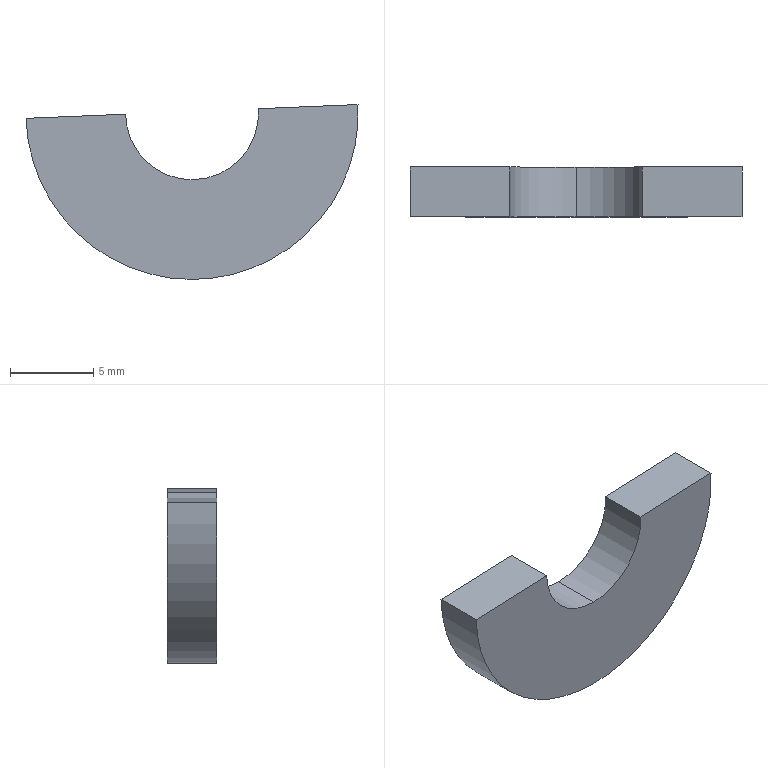Part | STEP file | Cuon T phu H01_8 | 1 solid | 8 faces | box 19.995 x 3 x 10.524 mm | volume 399.827 mm3 | cylinder 4 | plane 4 | commonest cylinder face diameters 8 x2 20 x2
STEP:
#1=CARTESIAN_POINT('',(0.,0.,0.));
#2=DIRECTION('',(0.,0.,1.));
#3=DIRECTION('',(1.,0.,0.));
#4=AXIS2_PLACEMENT_3D('',#1,#2,#3);
#5=CARTESIAN_POINT('',(3.99,3.,0.2758));
#6=VERTEX_POINT('',#5);
#7=CARTESIAN_POINT('',(3.99,0.,0.2758));
#8=VERTEX_POINT('',#7);
#9=CARTESIAN_POINT('',(3.99,3.,0.2758));
#10=DIRECTION('',(0.,-1.,0.));
#11=VECTOR('',#10,1.);
#12=LINE('',#9,#11);
#13=CARTESIAN_POINT('',(0.,3.,0.));
#14=DIRECTION('',(0.,-1.,0.));
#15=DIRECTION('',(0.,0.,-1.));
#16=AXIS2_PLACEMENT_3D('',#13,#14,#15);
#17=CYLINDRICAL_SURFACE('',#16,4.);
#18=CARTESIAN_POINT('',(1.64,0.));
#19=DIRECTION('',(0.,1.));
#20=VECTOR('',#19,1.);
#21=LINE('',#18,#20);
#22=(GEOMETRIC_REPRESENTATION_CONTEXT(2)PARAMETRIC_REPRESENTATION_CONTEXT()REPRESENTATION_CONTEXT('',''));
#23=DEFINITIONAL_REPRESENTATION('',(#21),#22);
#24=PCURVE('',#17,#23);
#25=CARTESIAN_POINT('',(-359.492,-20.57,-14.75));
#26=DIRECTION('',(0.0413,0.,-0.9991));
#27=DIRECTION('',(-0.9991,0.,-0.0413));
#28=AXIS2_PLACEMENT_3D('',#25,#26,#27);
#29=PLANE('',#28);
#30=CARTESIAN_POINT('',(-363.793,23.57));
#31=DIRECTION('',(0.,-1.));
#32=VECTOR('',#31,1.);
#33=LINE('',#30,#32);
#34=(GEOMETRIC_REPRESENTATION_CONTEXT(2)PARAMETRIC_REPRESENTATION_CONTEXT()REPRESENTATION_CONTEXT('',''));
#35=DEFINITIONAL_REPRESENTATION('',(#33),#34);
#36=PCURVE('',#29,#35);
#37=SURFACE_CURVE('',#12,(#24,#36),.PCURVE_S1.);
#38=EDGE_CURVE('',#6,#8,#37,.T.);
#39=ORIENTED_EDGE('',*,*,#38,.T.);
#40=CARTESIAN_POINT('',(0.,0.,-4.));
#41=VERTEX_POINT('',#40);
#42=CARTESIAN_POINT('',(0.,0.,0.));
#43=DIRECTION('',(0.,1.,0.));
#44=DIRECTION('',(0.,0.,1.));
#45=AXIS2_PLACEMENT_3D('',#42,#43,#44);
#46=CIRCLE('',#45,4.);
#47=CARTESIAN_POINT('',(3.142,3.));
#48=DIRECTION('',(-1.,0.));
#49=VECTOR('',#48,1.);
#50=LINE('',#47,#49);
#51=(GEOMETRIC_REPRESENTATION_CONTEXT(2)PARAMETRIC_REPRESENTATION_CONTEXT()REPRESENTATION_CONTEXT('',''));
#52=DEFINITIONAL_REPRESENTATION('',(#50),#51);
#53=PCURVE('',#17,#52);
#54=CARTESIAN_POINT('',(0.,0.,0.));
#55=DIRECTION('',(0.,1.,0.));
#56=DIRECTION('',(0.,0.,1.));
#57=AXIS2_PLACEMENT_3D('',#54,#55,#56);
#58=PLANE('',#57);
#59=CARTESIAN_POINT('',(0.,0.));
#60=DIRECTION('',(1.,0.));
#61=AXIS2_PLACEMENT_2D('',#59,#60);
#62=CIRCLE('',#61,4.);
#63=(GEOMETRIC_REPRESENTATION_CONTEXT(2)PARAMETRIC_REPRESENTATION_CONTEXT()REPRESENTATION_CONTEXT('',''));
#64=DEFINITIONAL_REPRESENTATION('',(#62),#63);
#65=PCURVE('',#58,#64);
#66=SURFACE_CURVE('',#46,(#53,#65),.PCURVE_S1.);
#67=EDGE_CURVE('',#8,#41,#66,.T.);
#68=ORIENTED_EDGE('',*,*,#67,.T.);
#69=CARTESIAN_POINT('',(0.,3.,-4.));
#70=VERTEX_POINT('',#69);
#71=CARTESIAN_POINT('',(0.,3.,-4.));
#72=DIRECTION('',(0.,-1.,0.));
#73=VECTOR('',#72,1.);
#74=LINE('',#71,#73);
#75=CARTESIAN_POINT('',(0.,0.));
#76=DIRECTION('',(0.,1.));
#77=VECTOR('',#76,1.);
#78=LINE('',#75,#77);
#79=(GEOMETRIC_REPRESENTATION_CONTEXT(2)PARAMETRIC_REPRESENTATION_CONTEXT()REPRESENTATION_CONTEXT('',''));
#80=DEFINITIONAL_REPRESENTATION('',(#78),#79);
#81=PCURVE('',#17,#80);
#82=CARTESIAN_POINT('',(0.,3.,0.));
#83=DIRECTION('',(0.,-1.,0.));
#84=DIRECTION('',(0.,0.,-1.));
#85=AXIS2_PLACEMENT_3D('',#82,#83,#84);
#86=CYLINDRICAL_SURFACE('',#85,4.);
#87=CARTESIAN_POINT('',(6.283,0.));
#88=DIRECTION('',(0.,1.));
#89=VECTOR('',#88,1.);
#90=LINE('',#87,#89);
#91=(GEOMETRIC_REPRESENTATION_CONTEXT(2)PARAMETRIC_REPRESENTATION_CONTEXT()REPRESENTATION_CONTEXT('',''));
#92=DEFINITIONAL_REPRESENTATION('',(#90),#91);
#93=PCURVE('',#86,#92);
#94=SURFACE_CURVE('',#74,(#81,#93),.PCURVE_S1.);
#95=EDGE_CURVE('',#70,#41,#94,.T.);
#96=ORIENTED_EDGE('',*,*,#95,.F.);
#97=CARTESIAN_POINT('',(0.,3.,0.));
#98=DIRECTION('',(0.,1.,0.));
#99=DIRECTION('',(0.,0.,1.));
#100=AXIS2_PLACEMENT_3D('',#97,#98,#99);
#101=CIRCLE('',#100,4.);
#102=CARTESIAN_POINT('',(3.142,0.));
#103=DIRECTION('',(-1.,0.));
#104=VECTOR('',#103,1.);
#105=LINE('',#102,#104);
#106=(GEOMETRIC_REPRESENTATION_CONTEXT(2)PARAMETRIC_REPRESENTATION_CONTEXT()REPRESENTATION_CONTEXT('',''));
#107=DEFINITIONAL_REPRESENTATION('',(#105),#106);
#108=PCURVE('',#17,#107);
#109=CARTESIAN_POINT('',(0.,3.,0.));
#110=DIRECTION('',(0.,1.,0.));
#111=DIRECTION('',(0.,0.,1.));
#112=AXIS2_PLACEMENT_3D('',#109,#110,#111);
#113=PLANE('',#112);
#114=CARTESIAN_POINT('',(0.,0.));
#115=DIRECTION('',(1.,0.));
#116=AXIS2_PLACEMENT_2D('',#114,#115);
#117=CIRCLE('',#116,4.);
#118=(GEOMETRIC_REPRESENTATION_CONTEXT(2)PARAMETRIC_REPRESENTATION_CONTEXT()REPRESENTATION_CONTEXT('',''));
#119=DEFINITIONAL_REPRESENTATION('',(#117),#118);
#120=PCURVE('',#113,#119);
#121=SURFACE_CURVE('',#101,(#108,#120),.PCURVE_S1.);
#122=EDGE_CURVE('',#6,#70,#121,.T.);
#123=ORIENTED_EDGE('',*,*,#122,.F.);
#124=EDGE_LOOP('',(#39,#68,#96,#123));
#125=FACE_BOUND('',#124,.F.);
#126=ADVANCED_FACE('',(#125),#17,.F.);
#127=CARTESIAN_POINT('',(0.,3.,-10.));
#128=VERTEX_POINT('',#127);
#129=CARTESIAN_POINT('',(-9.995,3.,-0.3024));
#130=VERTEX_POINT('',#129);
#131=CARTESIAN_POINT('',(0.,3.,0.));
#132=DIRECTION('',(0.,1.,0.));
#133=DIRECTION('',(0.,0.,1.));
#134=AXIS2_PLACEMENT_3D('',#131,#132,#133);
#135=CIRCLE('',#134,10.);
#136=CARTESIAN_POINT('',(0.,3.,0.));
#137=DIRECTION('',(0.,-1.,0.));
#138=DIRECTION('',(0.,0.,-1.));
#139=AXIS2_PLACEMENT_3D('',#136,#137,#138);
#140=CYLINDRICAL_SURFACE('',#139,10.);
#141=CARTESIAN_POINT('',(9.425,0.));
#142=DIRECTION('',(-1.,0.));
#143=VECTOR('',#142,1.);
#144=LINE('',#141,#143);
#145=(GEOMETRIC_REPRESENTATION_CONTEXT(2)PARAMETRIC_REPRESENTATION_CONTEXT()REPRESENTATION_CONTEXT('',''));
#146=DEFINITIONAL_REPRESENTATION('',(#144),#145);
#147=PCURVE('',#140,#146);
#148=CARTESIAN_POINT('',(0.,0.));
#149=DIRECTION('',(1.,0.));
#150=AXIS2_PLACEMENT_2D('',#148,#149);
#151=CIRCLE('',#150,10.);
#152=(GEOMETRIC_REPRESENTATION_CONTEXT(2)PARAMETRIC_REPRESENTATION_CONTEXT()REPRESENTATION_CONTEXT('',''));
#153=DEFINITIONAL_REPRESENTATION('',(#151),#152);
#154=PCURVE('',#113,#153);
#155=SURFACE_CURVE('',#135,(#147,#154),.PCURVE_S1.);
#156=EDGE_CURVE('',#128,#130,#155,.T.);
#157=ORIENTED_EDGE('',*,*,#156,.F.);
#158=CARTESIAN_POINT('',(0.,0.,-10.));
#159=VERTEX_POINT('',#158);
#160=CARTESIAN_POINT('',(0.,3.,-10.));
#161=DIRECTION('',(0.,-1.,0.));
#162=VECTOR('',#161,1.);
#163=LINE('',#160,#162);
#164=CARTESIAN_POINT('',(6.283,0.));
#165=DIRECTION('',(0.,1.));
#166=VECTOR('',#165,1.);
#167=LINE('',#164,#166);
#168=(GEOMETRIC_REPRESENTATION_CONTEXT(2)PARAMETRIC_REPRESENTATION_CONTEXT()REPRESENTATION_CONTEXT('',''));
#169=DEFINITIONAL_REPRESENTATION('',(#167),#168);
#170=PCURVE('',#140,#169);
#171=CARTESIAN_POINT('',(0.,3.,0.));
#172=DIRECTION('',(0.,-1.,0.));
#173=DIRECTION('',(0.,0.,-1.));
#174=AXIS2_PLACEMENT_3D('',#171,#172,#173);
#175=CYLINDRICAL_SURFACE('',#174,10.);
#176=CARTESIAN_POINT('',(0.,0.));
#177=DIRECTION('',(0.,1.));
#178=VECTOR('',#177,1.);
#179=LINE('',#176,#178);
#180=(GEOMETRIC_REPRESENTATION_CONTEXT(2)PARAMETRIC_REPRESENTATION_CONTEXT()REPRESENTATION_CONTEXT('',''));
#181=DEFINITIONAL_REPRESENTATION('',(#179),#180);
#182=PCURVE('',#175,#181);
#183=SURFACE_CURVE('',#163,(#170,#182),.PCURVE_S1.);
#184=EDGE_CURVE('',#128,#159,#183,.T.);
#185=ORIENTED_EDGE('',*,*,#184,.T.);
#186=CARTESIAN_POINT('',(-9.995,0.,-0.3024));
#187=VERTEX_POINT('',#186);
#188=CARTESIAN_POINT('',(0.,0.,0.));
#189=DIRECTION('',(0.,1.,0.));
#190=DIRECTION('',(0.,0.,1.));
#191=AXIS2_PLACEMENT_3D('',#188,#189,#190);
#192=CIRCLE('',#191,10.);
#193=CARTESIAN_POINT('',(9.425,3.));
#194=DIRECTION('',(-1.,0.));
#195=VECTOR('',#194,1.);
#196=LINE('',#193,#195);
#197=(GEOMETRIC_REPRESENTATION_CONTEXT(2)PARAMETRIC_REPRESENTATION_CONTEXT()REPRESENTATION_CONTEXT('',''));
#198=DEFINITIONAL_REPRESENTATION('',(#196),#197);
#199=PCURVE('',#140,#198);
#200=CARTESIAN_POINT('',(0.,0.));
#201=DIRECTION('',(1.,0.));
#202=AXIS2_PLACEMENT_2D('',#200,#201);
#203=CIRCLE('',#202,10.);
#204=(GEOMETRIC_REPRESENTATION_CONTEXT(2)PARAMETRIC_REPRESENTATION_CONTEXT()REPRESENTATION_CONTEXT('',''));
#205=DEFINITIONAL_REPRESENTATION('',(#203),#204);
#206=PCURVE('',#58,#205);
#207=SURFACE_CURVE('',#192,(#199,#206),.PCURVE_S1.);
#208=EDGE_CURVE('',#159,#187,#207,.T.);
#209=ORIENTED_EDGE('',*,*,#208,.T.);
#210=CARTESIAN_POINT('',(-9.995,3.,-0.3024));
#211=DIRECTION('',(0.,1.,0.));
#212=VECTOR('',#211,1.);
#213=LINE('',#210,#212);
#214=CARTESIAN_POINT('',(4.743,0.));
#215=DIRECTION('',(0.,-1.));
#216=VECTOR('',#215,1.);
#217=LINE('',#214,#216);
#218=(GEOMETRIC_REPRESENTATION_CONTEXT(2)PARAMETRIC_REPRESENTATION_CONTEXT()REPRESENTATION_CONTEXT('',''));
#219=DEFINITIONAL_REPRESENTATION('',(#217),#218);
#220=PCURVE('',#140,#219);
#221=CARTESIAN_POINT('',(-359.492,-20.57,-14.75));
#222=DIRECTION('',(0.0413,0.,-0.9991));
#223=DIRECTION('',(-0.9991,0.,-0.0413));
#224=AXIS2_PLACEMENT_3D('',#221,#222,#223);
#225=PLANE('',#224);
#226=CARTESIAN_POINT('',(-349.795,23.57));
#227=DIRECTION('',(0.,1.));
#228=VECTOR('',#227,1.);
#229=LINE('',#226,#228);
#230=(GEOMETRIC_REPRESENTATION_CONTEXT(2)PARAMETRIC_REPRESENTATION_CONTEXT()REPRESENTATION_CONTEXT('',''));
#231=DEFINITIONAL_REPRESENTATION('',(#229),#230);
#232=PCURVE('',#225,#231);
#233=SURFACE_CURVE('',#213,(#220,#232),.PCURVE_S1.);
#234=EDGE_CURVE('',#187,#130,#233,.T.);
#235=ORIENTED_EDGE('',*,*,#234,.T.);
#236=EDGE_LOOP('',(#157,#185,#209,#235));
#237=FACE_BOUND('',#236,.T.);
#238=ADVANCED_FACE('',(#237),#140,.T.);
#239=CARTESIAN_POINT('',(9.986,3.,0.5237));
#240=VERTEX_POINT('',#239);
#241=CARTESIAN_POINT('',(-0.004574,3.,0.1106));
#242=DIRECTION('',(-0.9991,0.,-0.0413));
#243=VECTOR('',#242,1.);
#244=LINE('',#241,#243);
#245=CARTESIAN_POINT('',(0.1106,-0.004574));
#246=DIRECTION('',(-0.0413,-0.9991));
#247=VECTOR('',#246,1.);
#248=LINE('',#245,#247);
#249=(GEOMETRIC_REPRESENTATION_CONTEXT(2)PARAMETRIC_REPRESENTATION_CONTEXT()REPRESENTATION_CONTEXT('',''));
#250=DEFINITIONAL_REPRESENTATION('',(#248),#249);
#251=PCURVE('',#113,#250);
#252=CARTESIAN_POINT('',(-359.795,23.57));
#253=DIRECTION('',(1.,0.));
#254=VECTOR('',#253,1.);
#255=LINE('',#252,#254);
#256=(GEOMETRIC_REPRESENTATION_CONTEXT(2)PARAMETRIC_REPRESENTATION_CONTEXT()REPRESENTATION_CONTEXT('',''));
#257=DEFINITIONAL_REPRESENTATION('',(#255),#256);
#258=PCURVE('',#29,#257);
#259=SURFACE_CURVE('',#244,(#251,#258),.PCURVE_S1.);
#260=EDGE_CURVE('',#240,#6,#259,.T.);
#261=ORIENTED_EDGE('',*,*,#260,.F.);
#262=CARTESIAN_POINT('',(0.,3.,0.));
#263=DIRECTION('',(0.,1.,0.));
#264=DIRECTION('',(0.,0.,1.));
#265=AXIS2_PLACEMENT_3D('',#262,#263,#264);
#266=CIRCLE('',#265,10.);
#267=CARTESIAN_POINT('',(0.,0.));
#268=DIRECTION('',(1.,0.));
#269=AXIS2_PLACEMENT_2D('',#267,#268);
#270=CIRCLE('',#269,10.);
#271=(GEOMETRIC_REPRESENTATION_CONTEXT(2)PARAMETRIC_REPRESENTATION_CONTEXT()REPRESENTATION_CONTEXT('',''));
#272=DEFINITIONAL_REPRESENTATION('',(#270),#271);
#273=PCURVE('',#113,#272);
#274=CARTESIAN_POINT('',(3.142,0.));
#275=DIRECTION('',(-1.,0.));
#276=VECTOR('',#275,1.);
#277=LINE('',#274,#276);
#278=(GEOMETRIC_REPRESENTATION_CONTEXT(2)PARAMETRIC_REPRESENTATION_CONTEXT()REPRESENTATION_CONTEXT('',''));
#279=DEFINITIONAL_REPRESENTATION('',(#277),#278);
#280=PCURVE('',#175,#279);
#281=SURFACE_CURVE('',#266,(#273,#280),.PCURVE_S1.);
#282=EDGE_CURVE('',#240,#128,#281,.T.);
#283=ORIENTED_EDGE('',*,*,#282,.T.);
#284=ORIENTED_EDGE('',*,*,#156,.T.);
#285=CARTESIAN_POINT('',(-4.,3.,-0.05451));
#286=VERTEX_POINT('',#285);
#287=CARTESIAN_POINT('',(-0.004574,3.,0.1106));
#288=DIRECTION('',(-0.9991,0.,-0.0413));
#289=VECTOR('',#288,1.);
#290=LINE('',#287,#289);
#291=CARTESIAN_POINT('',(0.1106,-0.004574));
#292=DIRECTION('',(-0.0413,-0.9991));
#293=VECTOR('',#292,1.);
#294=LINE('',#291,#293);
#295=(GEOMETRIC_REPRESENTATION_CONTEXT(2)PARAMETRIC_REPRESENTATION_CONTEXT()REPRESENTATION_CONTEXT('',''));
#296=DEFINITIONAL_REPRESENTATION('',(#294),#295);
#297=PCURVE('',#113,#296);
#298=CARTESIAN_POINT('',(-359.795,23.57));
#299=DIRECTION('',(1.,0.));
#300=VECTOR('',#299,1.);
#301=LINE('',#298,#300);
#302=(GEOMETRIC_REPRESENTATION_CONTEXT(2)PARAMETRIC_REPRESENTATION_CONTEXT()REPRESENTATION_CONTEXT('',''));
#303=DEFINITIONAL_REPRESENTATION('',(#301),#302);
#304=PCURVE('',#225,#303);
#305=SURFACE_CURVE('',#290,(#297,#304),.PCURVE_S1.);
#306=EDGE_CURVE('',#286,#130,#305,.T.);
#307=ORIENTED_EDGE('',*,*,#306,.F.);
#308=CARTESIAN_POINT('',(0.,3.,0.));
#309=DIRECTION('',(0.,1.,0.));
#310=DIRECTION('',(0.,0.,1.));
#311=AXIS2_PLACEMENT_3D('',#308,#309,#310);
#312=CIRCLE('',#311,4.);
#313=CARTESIAN_POINT('',(0.,0.));
#314=DIRECTION('',(1.,0.));
#315=AXIS2_PLACEMENT_2D('',#313,#314);
#316=CIRCLE('',#315,4.);
#317=(GEOMETRIC_REPRESENTATION_CONTEXT(2)PARAMETRIC_REPRESENTATION_CONTEXT()REPRESENTATION_CONTEXT('',''));
#318=DEFINITIONAL_REPRESENTATION('',(#316),#317);
#319=PCURVE('',#113,#318);
#320=CARTESIAN_POINT('',(9.425,0.));
#321=DIRECTION('',(-1.,0.));
#322=VECTOR('',#321,1.);
#323=LINE('',#320,#322);
#324=(GEOMETRIC_REPRESENTATION_CONTEXT(2)PARAMETRIC_REPRESENTATION_CONTEXT()REPRESENTATION_CONTEXT('',''));
#325=DEFINITIONAL_REPRESENTATION('',(#323),#324);
#326=PCURVE('',#86,#325);
#327=SURFACE_CURVE('',#312,(#319,#326),.PCURVE_S1.);
#328=EDGE_CURVE('',#70,#286,#327,.T.);
#329=ORIENTED_EDGE('',*,*,#328,.F.);
#330=ORIENTED_EDGE('',*,*,#122,.F.);
#331=EDGE_LOOP('',(#261,#283,#284,#307,#329,#330));
#332=FACE_BOUND('',#331,.T.);
#333=ADVANCED_FACE('',(#332),#113,.T.);
#334=CARTESIAN_POINT('',(9.986,0.,0.5237));
#335=VERTEX_POINT('',#334);
#336=CARTESIAN_POINT('',(0.,0.,0.));
#337=DIRECTION('',(0.,1.,0.));
#338=DIRECTION('',(0.,0.,1.));
#339=AXIS2_PLACEMENT_3D('',#336,#337,#338);
#340=CIRCLE('',#339,10.);
#341=CARTESIAN_POINT('',(0.,0.));
#342=DIRECTION('',(1.,0.));
#343=AXIS2_PLACEMENT_2D('',#341,#342);
#344=CIRCLE('',#343,10.);
#345=(GEOMETRIC_REPRESENTATION_CONTEXT(2)PARAMETRIC_REPRESENTATION_CONTEXT()REPRESENTATION_CONTEXT('',''));
#346=DEFINITIONAL_REPRESENTATION('',(#344),#345);
#347=PCURVE('',#58,#346);
#348=CARTESIAN_POINT('',(3.142,3.));
#349=DIRECTION('',(-1.,0.));
#350=VECTOR('',#349,1.);
#351=LINE('',#348,#350);
#352=(GEOMETRIC_REPRESENTATION_CONTEXT(2)PARAMETRIC_REPRESENTATION_CONTEXT()REPRESENTATION_CONTEXT('',''));
#353=DEFINITIONAL_REPRESENTATION('',(#351),#352);
#354=PCURVE('',#175,#353);
#355=SURFACE_CURVE('',#340,(#347,#354),.PCURVE_S1.);
#356=EDGE_CURVE('',#335,#159,#355,.T.);
#357=ORIENTED_EDGE('',*,*,#356,.F.);
#358=CARTESIAN_POINT('',(-0.004574,0.,0.1106));
#359=DIRECTION('',(-0.9991,0.,-0.0413));
#360=VECTOR('',#359,1.);
#361=LINE('',#358,#360);
#362=CARTESIAN_POINT('',(0.1106,-0.004574));
#363=DIRECTION('',(-0.0413,-0.9991));
#364=VECTOR('',#363,1.);
#365=LINE('',#362,#364);
#366=(GEOMETRIC_REPRESENTATION_CONTEXT(2)PARAMETRIC_REPRESENTATION_CONTEXT()REPRESENTATION_CONTEXT('',''));
#367=DEFINITIONAL_REPRESENTATION('',(#365),#366);
#368=PCURVE('',#58,#367);
#369=CARTESIAN_POINT('',(-359.795,20.57));
#370=DIRECTION('',(1.,0.));
#371=VECTOR('',#370,1.);
#372=LINE('',#369,#371);
#373=(GEOMETRIC_REPRESENTATION_CONTEXT(2)PARAMETRIC_REPRESENTATION_CONTEXT()REPRESENTATION_CONTEXT('',''));
#374=DEFINITIONAL_REPRESENTATION('',(#372),#373);
#375=PCURVE('',#29,#374);
#376=SURFACE_CURVE('',#361,(#368,#375),.PCURVE_S1.);
#377=EDGE_CURVE('',#335,#8,#376,.T.);
#378=ORIENTED_EDGE('',*,*,#377,.T.);
#379=ORIENTED_EDGE('',*,*,#67,.T.);
#380=CARTESIAN_POINT('',(-4.,0.,-0.05451));
#381=VERTEX_POINT('',#380);
#382=CARTESIAN_POINT('',(0.,0.,0.));
#383=DIRECTION('',(0.,1.,0.));
#384=DIRECTION('',(0.,0.,1.));
#385=AXIS2_PLACEMENT_3D('',#382,#383,#384);
#386=CIRCLE('',#385,4.);
#387=CARTESIAN_POINT('',(0.,0.));
#388=DIRECTION('',(1.,0.));
#389=AXIS2_PLACEMENT_2D('',#387,#388);
#390=CIRCLE('',#389,4.);
#391=(GEOMETRIC_REPRESENTATION_CONTEXT(2)PARAMETRIC_REPRESENTATION_CONTEXT()REPRESENTATION_CONTEXT('',''));
#392=DEFINITIONAL_REPRESENTATION('',(#390),#391);
#393=PCURVE('',#58,#392);
#394=CARTESIAN_POINT('',(9.425,3.));
#395=DIRECTION('',(-1.,0.));
#396=VECTOR('',#395,1.);
#397=LINE('',#394,#396);
#398=(GEOMETRIC_REPRESENTATION_CONTEXT(2)PARAMETRIC_REPRESENTATION_CONTEXT()REPRESENTATION_CONTEXT('',''));
#399=DEFINITIONAL_REPRESENTATION('',(#397),#398);
#400=PCURVE('',#86,#399);
#401=SURFACE_CURVE('',#386,(#393,#400),.PCURVE_S1.);
#402=EDGE_CURVE('',#41,#381,#401,.T.);
#403=ORIENTED_EDGE('',*,*,#402,.T.);
#404=CARTESIAN_POINT('',(-0.004574,0.,0.1106));
#405=DIRECTION('',(-0.9991,0.,-0.0413));
#406=VECTOR('',#405,1.);
#407=LINE('',#404,#406);
#408=CARTESIAN_POINT('',(0.1106,-0.004574));
#409=DIRECTION('',(-0.0413,-0.9991));
#410=VECTOR('',#409,1.);
#411=LINE('',#408,#410);
#412=(GEOMETRIC_REPRESENTATION_CONTEXT(2)PARAMETRIC_REPRESENTATION_CONTEXT()REPRESENTATION_CONTEXT('',''));
#413=DEFINITIONAL_REPRESENTATION('',(#411),#412);
#414=PCURVE('',#58,#413);
#415=CARTESIAN_POINT('',(-359.795,20.57));
#416=DIRECTION('',(1.,0.));
#417=VECTOR('',#416,1.);
#418=LINE('',#415,#417);
#419=(GEOMETRIC_REPRESENTATION_CONTEXT(2)PARAMETRIC_REPRESENTATION_CONTEXT()REPRESENTATION_CONTEXT('',''));
#420=DEFINITIONAL_REPRESENTATION('',(#418),#419);
#421=PCURVE('',#225,#420);
#422=SURFACE_CURVE('',#407,(#414,#421),.PCURVE_S1.);
#423=EDGE_CURVE('',#381,#187,#422,.T.);
#424=ORIENTED_EDGE('',*,*,#423,.T.);
#425=ORIENTED_EDGE('',*,*,#208,.F.);
#426=EDGE_LOOP('',(#357,#378,#379,#403,#424,#425));
#427=FACE_BOUND('',#426,.T.);
#428=ADVANCED_FACE('',(#427),#58,.F.);
#429=ORIENTED_EDGE('',*,*,#184,.F.);
#430=ORIENTED_EDGE('',*,*,#282,.F.);
#431=CARTESIAN_POINT('',(9.986,3.,0.5237));
#432=DIRECTION('',(0.,-1.,0.));
#433=VECTOR('',#432,1.);
#434=LINE('',#431,#433);
#435=CARTESIAN_POINT('',(1.623,0.));
#436=DIRECTION('',(0.,1.));
#437=VECTOR('',#436,1.);
#438=LINE('',#435,#437);
#439=(GEOMETRIC_REPRESENTATION_CONTEXT(2)PARAMETRIC_REPRESENTATION_CONTEXT()REPRESENTATION_CONTEXT('',''));
#440=DEFINITIONAL_REPRESENTATION('',(#438),#439);
#441=PCURVE('',#175,#440);
#442=CARTESIAN_POINT('',(-369.794,23.57));
#443=DIRECTION('',(0.,-1.));
#444=VECTOR('',#443,1.);
#445=LINE('',#442,#444);
#446=(GEOMETRIC_REPRESENTATION_CONTEXT(2)PARAMETRIC_REPRESENTATION_CONTEXT()REPRESENTATION_CONTEXT('',''));
#447=DEFINITIONAL_REPRESENTATION('',(#445),#446);
#448=PCURVE('',#29,#447);
#449=SURFACE_CURVE('',#434,(#441,#448),.PCURVE_S1.);
#450=EDGE_CURVE('',#240,#335,#449,.T.);
#451=ORIENTED_EDGE('',*,*,#450,.T.);
#452=ORIENTED_EDGE('',*,*,#356,.T.);
#453=EDGE_LOOP('',(#429,#430,#451,#452));
#454=FACE_BOUND('',#453,.T.);
#455=ADVANCED_FACE('',(#454),#175,.T.);
#456=ORIENTED_EDGE('',*,*,#402,.T.);
#457=CARTESIAN_POINT('',(-4.,3.,-0.05451));
#458=DIRECTION('',(0.,1.,0.));
#459=VECTOR('',#458,1.);
#460=LINE('',#457,#459);
#461=CARTESIAN_POINT('',(4.726,0.));
#462=DIRECTION('',(0.,-1.));
#463=VECTOR('',#462,1.);
#464=LINE('',#461,#463);
#465=(GEOMETRIC_REPRESENTATION_CONTEXT(2)PARAMETRIC_REPRESENTATION_CONTEXT()REPRESENTATION_CONTEXT('',''));
#466=DEFINITIONAL_REPRESENTATION('',(#464),#465);
#467=PCURVE('',#86,#466);
#468=CARTESIAN_POINT('',(-355.796,23.57));
#469=DIRECTION('',(0.,1.));
#470=VECTOR('',#469,1.);
#471=LINE('',#468,#470);
#472=(GEOMETRIC_REPRESENTATION_CONTEXT(2)PARAMETRIC_REPRESENTATION_CONTEXT()REPRESENTATION_CONTEXT('',''));
#473=DEFINITIONAL_REPRESENTATION('',(#471),#472);
#474=PCURVE('',#225,#473);
#475=SURFACE_CURVE('',#460,(#467,#474),.PCURVE_S1.);
#476=EDGE_CURVE('',#381,#286,#475,.T.);
#477=ORIENTED_EDGE('',*,*,#476,.T.);
#478=ORIENTED_EDGE('',*,*,#328,.F.);
#479=ORIENTED_EDGE('',*,*,#95,.T.);
#480=EDGE_LOOP('',(#456,#477,#478,#479));
#481=FACE_BOUND('',#480,.F.);
#482=ADVANCED_FACE('',(#481),#86,.F.);
#483=ORIENTED_EDGE('',*,*,#423,.F.);
#484=ORIENTED_EDGE('',*,*,#476,.T.);
#485=ORIENTED_EDGE('',*,*,#306,.T.);
#486=ORIENTED_EDGE('',*,*,#234,.F.);
#487=EDGE_LOOP('',(#483,#484,#485,#486));
#488=FACE_BOUND('',#487,.T.);
#489=ADVANCED_FACE('',(#488),#225,.F.);
#490=ORIENTED_EDGE('',*,*,#260,.T.);
#491=ORIENTED_EDGE('',*,*,#38,.T.);
#492=ORIENTED_EDGE('',*,*,#377,.F.);
#493=ORIENTED_EDGE('',*,*,#450,.F.);
#494=EDGE_LOOP('',(#490,#491,#492,#493));
#495=FACE_BOUND('',#494,.T.);
#496=ADVANCED_FACE('',(#495),#29,.F.);
#497=CLOSED_SHELL('',(#126,#238,#333,#428,#455,#482,#489,#496));
#498=MANIFOLD_SOLID_BREP('',#497);
#499=(LENGTH_UNIT()NAMED_UNIT(*)SI_UNIT(.MILLI.,.METRE.));
#500=UNCERTAINTY_MEASURE_WITH_UNIT(LENGTH_MEASURE(0.0000001),#499,'','');
#501=(NAMED_UNIT(*)PLANE_ANGLE_UNIT()SI_UNIT($,.RADIAN.));
#502=(NAMED_UNIT(*)SI_UNIT($,.STERADIAN.)SOLID_ANGLE_UNIT());
#503=(GEOMETRIC_REPRESENTATION_CONTEXT(3)GLOBAL_UNCERTAINTY_ASSIGNED_CONTEXT((#500))GLOBAL_UNIT_ASSIGNED_CONTEXT((#499,#501,#502))REPRESENTATION_CONTEXT('',''));
#504=ADVANCED_BREP_SHAPE_REPRESENTATION('',(#4,#498),#503);